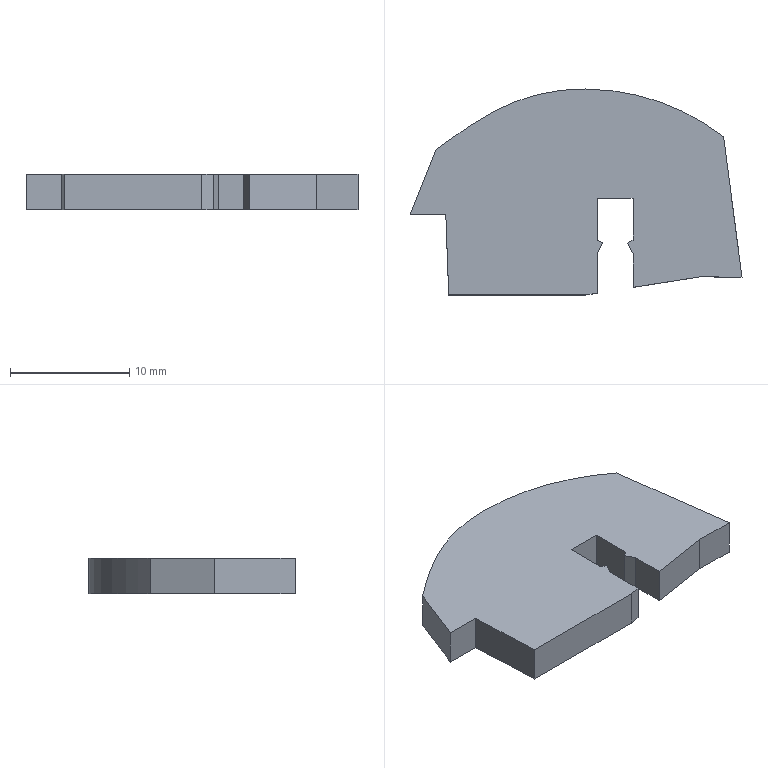Part | SolidWorks | features BaseBody 1 | 1 solid | 21 faces | box 27.839 x 17.276 x 3 mm | volume 1069 mm3 | plane 13 | spline 8
STEP:
#1=CARTESIAN_POINT('',(9.27,15.287,-1.5));
#2=VERTEX_POINT('',#1);
#3=CARTESIAN_POINT('',(-0.006107,19.138,-1.5));
#4=VERTEX_POINT('',#3);
#5=CARTESIAN_POINT('',(9.27,15.287,-1.5));
#6=CARTESIAN_POINT('',(6.696,17.285,-1.5));
#7=CARTESIAN_POINT('',(3.539,18.688,-1.5));
#8=CARTESIAN_POINT('',(-0.006107,19.138,-1.5));
#9=B_SPLINE_CURVE_WITH_KNOTS('',3,(#5,#6,#7,#8),.UNSPECIFIED.,.F.,.F.,(4,4),(0.9,1.),.UNSPECIFIED.);
#10=EDGE_CURVE('',#2,#4,#9,.T.);
#11=ORIENTED_EDGE('',*,*,#10,.F.);
#12=CARTESIAN_POINT('',(10.816,3.504,-1.5));
#13=VERTEX_POINT('',#12);
#14=CARTESIAN_POINT('',(10.816,3.504,-1.5));
#15=CARTESIAN_POINT('',(9.799,11.355,-1.5));
#16=CARTESIAN_POINT('',(9.27,15.287,-1.5));
#17=B_SPLINE_CURVE_WITH_KNOTS('',2,(#14,#15,#16),.UNSPECIFIED.,.F.,.F.,(3,3),(0.85,0.9),.UNSPECIFIED.);
#18=EDGE_CURVE('',#13,#2,#17,.T.);
#19=ORIENTED_EDGE('',*,*,#18,.F.);
#20=CARTESIAN_POINT('',(7.333,3.55,-1.5));
#21=VERTEX_POINT('',#20);
#22=CARTESIAN_POINT('',(7.333,3.55,-1.5));
#23=CARTESIAN_POINT('',(8.52,3.533,-1.5));
#24=CARTESIAN_POINT('',(10.816,3.504,-1.5));
#25=B_SPLINE_CURVE_WITH_KNOTS('',2,(#22,#23,#24),.UNSPECIFIED.,.F.,.F.,(3,3),(0.8,0.85),.UNSPECIFIED.);
#26=EDGE_CURVE('',#21,#13,#25,.T.);
#27=ORIENTED_EDGE('',*,*,#26,.F.);
#28=CARTESIAN_POINT('',(1.678,2.665,-1.5));
#29=VERTEX_POINT('',#28);
#30=CARTESIAN_POINT('',(1.678,2.665,-1.5));
#31=CARTESIAN_POINT('',(5.448,3.256,-1.5));
#32=CARTESIAN_POINT('',(7.333,3.55,-1.5));
#33=B_SPLINE_CURVE_WITH_KNOTS('',2,(#30,#31,#32),.UNSPECIFIED.,.F.,.F.,(3,3),(0.75,0.8),.UNSPECIFIED.);
#34=EDGE_CURVE('',#29,#21,#33,.T.);
#35=ORIENTED_EDGE('',*,*,#34,.F.);
#36=CARTESIAN_POINT('',(1.678,5.468,-1.5));
#37=VERTEX_POINT('',#36);
#38=CARTESIAN_POINT('',(1.678,5.468,-1.5));
#39=DIRECTION('',(0.,-1.,0.));
#40=VECTOR('',#39,1000.);
#41=LINE('',#38,#40);
#42=EDGE_CURVE('',#37,#29,#41,.T.);
#43=ORIENTED_EDGE('',*,*,#42,.F.);
#44=CARTESIAN_POINT('',(1.228,6.361,-1.5));
#45=VERTEX_POINT('',#44);
#46=CARTESIAN_POINT('',(1.228,6.361,-1.5));
#47=DIRECTION('',(0.4506,-0.8927,0.));
#48=VECTOR('',#47,1000.);
#49=LINE('',#46,#48);
#50=EDGE_CURVE('',#45,#37,#49,.T.);
#51=ORIENTED_EDGE('',*,*,#50,.F.);
#52=CARTESIAN_POINT('',(1.678,6.624,-1.5));
#53=VERTEX_POINT('',#52);
#54=CARTESIAN_POINT('',(1.678,6.624,-1.5));
#55=DIRECTION('',(-0.8634,-0.5045,0.));
#56=VECTOR('',#55,1000.);
#57=LINE('',#54,#56);
#58=EDGE_CURVE('',#53,#45,#57,.T.);
#59=ORIENTED_EDGE('',*,*,#58,.F.);
#60=CARTESIAN_POINT('',(1.678,10.134,-1.5));
#61=VERTEX_POINT('',#60);
#62=CARTESIAN_POINT('',(1.678,10.134,-1.5));
#63=DIRECTION('',(0.,-1.,0.));
#64=VECTOR('',#63,1000.);
#65=LINE('',#62,#64);
#66=EDGE_CURVE('',#61,#53,#65,.T.);
#67=ORIENTED_EDGE('',*,*,#66,.F.);
#68=CARTESIAN_POINT('',(-1.319,10.134,-1.5));
#69=VERTEX_POINT('',#68);
#70=CARTESIAN_POINT('',(-1.319,10.134,-1.5));
#71=DIRECTION('',(1.,0.,0.));
#72=VECTOR('',#71,1000.);
#73=LINE('',#70,#72);
#74=EDGE_CURVE('',#69,#61,#73,.T.);
#75=ORIENTED_EDGE('',*,*,#74,.F.);
#76=CARTESIAN_POINT('',(-1.319,6.624,-1.5));
#77=VERTEX_POINT('',#76);
#78=CARTESIAN_POINT('',(-1.319,6.624,-1.5));
#79=DIRECTION('',(0.,1.,0.));
#80=VECTOR('',#79,1000.);
#81=LINE('',#78,#80);
#82=EDGE_CURVE('',#77,#69,#81,.T.);
#83=ORIENTED_EDGE('',*,*,#82,.F.);
#84=CARTESIAN_POINT('',(-0.8705,6.393,-1.5));
#85=VERTEX_POINT('',#84);
#86=CARTESIAN_POINT('',(-0.8705,6.393,-1.5));
#87=DIRECTION('',(-0.8897,0.4565,0.));
#88=VECTOR('',#87,1000.);
#89=LINE('',#86,#88);
#90=EDGE_CURVE('',#85,#77,#89,.T.);
#91=ORIENTED_EDGE('',*,*,#90,.F.);
#92=CARTESIAN_POINT('',(-1.319,5.468,-1.5));
#93=VERTEX_POINT('',#92);
#94=CARTESIAN_POINT('',(-1.319,5.468,-1.5));
#95=DIRECTION('',(0.4365,0.8997,0.));
#96=VECTOR('',#95,1000.);
#97=LINE('',#94,#96);
#98=EDGE_CURVE('',#93,#85,#97,.T.);
#99=ORIENTED_EDGE('',*,*,#98,.F.);
#100=CARTESIAN_POINT('',(-1.319,2.18,-1.5));
#101=VERTEX_POINT('',#100);
#102=CARTESIAN_POINT('',(-1.319,2.18,-1.5));
#103=DIRECTION('',(0.,1.,0.));
#104=VECTOR('',#103,1000.);
#105=LINE('',#102,#104);
#106=EDGE_CURVE('',#101,#93,#105,.T.);
#107=ORIENTED_EDGE('',*,*,#106,.F.);
#108=CARTESIAN_POINT('',(-2.279,2.022,-1.5));
#109=VERTEX_POINT('',#108);
#110=CARTESIAN_POINT('',(-2.279,2.022,-1.5));
#111=CARTESIAN_POINT('',(-1.959,2.076,-1.5));
#112=CARTESIAN_POINT('',(-1.319,2.18,-1.5));
#113=B_SPLINE_CURVE_WITH_KNOTS('',2,(#110,#111,#112),.UNSPECIFIED.,.F.,.F.,(3,3),(0.25,0.3),.UNSPECIFIED.);
#114=EDGE_CURVE('',#109,#101,#113,.T.);
#115=ORIENTED_EDGE('',*,*,#114,.F.);
#116=CARTESIAN_POINT('',(-13.778,2.022,-1.5));
#117=VERTEX_POINT('',#116);
#118=CARTESIAN_POINT('',(-13.778,2.022,-1.5));
#119=DIRECTION('',(1.,0.,0.));
#120=VECTOR('',#119,1000.);
#121=LINE('',#118,#120);
#122=EDGE_CURVE('',#117,#109,#121,.T.);
#123=ORIENTED_EDGE('',*,*,#122,.F.);
#124=CARTESIAN_POINT('',(-14.022,8.734,-1.5));
#125=VERTEX_POINT('',#124);
#126=CARTESIAN_POINT('',(-14.022,8.734,-1.5));
#127=CARTESIAN_POINT('',(-13.939,6.499,-1.5));
#128=CARTESIAN_POINT('',(-13.858,4.261,-1.5));
#129=CARTESIAN_POINT('',(-13.778,2.022,-1.5));
#130=B_SPLINE_CURVE_WITH_KNOTS('',3,(#126,#127,#128,#129),.UNSPECIFIED.,.F.,.F.,(4,4),(0.15,0.2),.UNSPECIFIED.);
#131=EDGE_CURVE('',#125,#117,#130,.T.);
#132=ORIENTED_EDGE('',*,*,#131,.F.);
#133=CARTESIAN_POINT('',(-17.024,8.734,-1.5));
#134=VERTEX_POINT('',#133);
#135=CARTESIAN_POINT('',(-17.024,8.734,-1.5));
#136=DIRECTION('',(1.,0.,0.));
#137=VECTOR('',#136,1000.);
#138=LINE('',#135,#137);
#139=EDGE_CURVE('',#134,#125,#138,.T.);
#140=ORIENTED_EDGE('',*,*,#139,.F.);
#141=CARTESIAN_POINT('',(-14.868,14.173,-1.5));
#142=VERTEX_POINT('',#141);
#143=CARTESIAN_POINT('',(-14.868,14.173,-1.5));
#144=CARTESIAN_POINT('',(-15.587,12.359,-1.5));
#145=CARTESIAN_POINT('',(-16.305,10.548,-1.5));
#146=CARTESIAN_POINT('',(-17.024,8.734,-1.5));
#147=B_SPLINE_CURVE_WITH_KNOTS('',3,(#143,#144,#145,#146),.UNSPECIFIED.,.F.,.F.,(4,4),(0.05,0.1),.UNSPECIFIED.);
#148=EDGE_CURVE('',#142,#134,#147,.T.);
#149=ORIENTED_EDGE('',*,*,#148,.F.);
#150=CARTESIAN_POINT('',(-0.006107,19.138,-1.5));
#151=CARTESIAN_POINT('',(-6.949,20.02,-1.5));
#152=CARTESIAN_POINT('',(-10.909,17.098,-1.5));
#153=CARTESIAN_POINT('',(-14.868,14.173,-1.5));
#154=B_SPLINE_CURVE_WITH_KNOTS('',3,(#150,#151,#152,#153),.UNSPECIFIED.,.F.,.F.,(4,4),(0.,0.05),.UNSPECIFIED.);
#155=EDGE_CURVE('',#4,#142,#154,.T.);
#156=ORIENTED_EDGE('',*,*,#155,.F.);
#157=EDGE_LOOP('',(#11,#19,#27,#35,#43,#51,#59,#67,#75,#83,#91,#99,#107,#115,#123,#132,#140,#149,#156));
#158=FACE_OUTER_BOUND('',#157,.T.);
#159=CARTESIAN_POINT('',(4.996,17.793,-1.5));
#160=DIRECTION('',(0.,0.,-1.));
#161=DIRECTION('',(0.,-1.,0.));
#162=AXIS2_PLACEMENT_3D('',#159,#160,#161);
#163=PLANE('',#162);
#164=ADVANCED_FACE('',(#158),#163,.T.);
#165=CARTESIAN_POINT('',(9.27,15.287,1.5));
#166=VERTEX_POINT('',#165);
#167=CARTESIAN_POINT('',(-0.006107,19.138,1.5));
#168=VERTEX_POINT('',#167);
#169=CARTESIAN_POINT('',(9.27,15.287,1.5));
#170=CARTESIAN_POINT('',(6.696,17.285,1.5));
#171=CARTESIAN_POINT('',(3.539,18.688,1.5));
#172=CARTESIAN_POINT('',(-0.006107,19.138,1.5));
#173=B_SPLINE_CURVE_WITH_KNOTS('',3,(#169,#170,#171,#172),.UNSPECIFIED.,.F.,.F.,(4,4),(0.9,1.),.UNSPECIFIED.);
#174=EDGE_CURVE('',#166,#168,#173,.T.);
#175=ORIENTED_EDGE('',*,*,#174,.T.);
#176=CARTESIAN_POINT('',(-14.868,14.173,1.5));
#177=VERTEX_POINT('',#176);
#178=CARTESIAN_POINT('',(-0.006107,19.138,1.5));
#179=CARTESIAN_POINT('',(-6.949,20.02,1.5));
#180=CARTESIAN_POINT('',(-10.909,17.098,1.5));
#181=CARTESIAN_POINT('',(-14.868,14.173,1.5));
#182=B_SPLINE_CURVE_WITH_KNOTS('',3,(#178,#179,#180,#181),.UNSPECIFIED.,.F.,.F.,(4,4),(0.,0.05),.UNSPECIFIED.);
#183=EDGE_CURVE('',#168,#177,#182,.T.);
#184=ORIENTED_EDGE('',*,*,#183,.T.);
#185=CARTESIAN_POINT('',(-17.024,8.734,1.5));
#186=VERTEX_POINT('',#185);
#187=CARTESIAN_POINT('',(-14.868,14.173,1.5));
#188=CARTESIAN_POINT('',(-15.587,12.359,1.5));
#189=CARTESIAN_POINT('',(-16.305,10.548,1.5));
#190=CARTESIAN_POINT('',(-17.024,8.734,1.5));
#191=B_SPLINE_CURVE_WITH_KNOTS('',3,(#187,#188,#189,#190),.UNSPECIFIED.,.F.,.F.,(4,4),(0.05,0.1),.UNSPECIFIED.);
#192=EDGE_CURVE('',#177,#186,#191,.T.);
#193=ORIENTED_EDGE('',*,*,#192,.T.);
#194=CARTESIAN_POINT('',(-14.022,8.734,1.5));
#195=VERTEX_POINT('',#194);
#196=CARTESIAN_POINT('',(-17.024,8.734,1.5));
#197=DIRECTION('',(1.,0.,0.));
#198=VECTOR('',#197,1000.);
#199=LINE('',#196,#198);
#200=EDGE_CURVE('',#186,#195,#199,.T.);
#201=ORIENTED_EDGE('',*,*,#200,.T.);
#202=CARTESIAN_POINT('',(-13.778,2.022,1.5));
#203=VERTEX_POINT('',#202);
#204=CARTESIAN_POINT('',(-14.022,8.734,1.5));
#205=CARTESIAN_POINT('',(-13.939,6.499,1.5));
#206=CARTESIAN_POINT('',(-13.858,4.261,1.5));
#207=CARTESIAN_POINT('',(-13.778,2.022,1.5));
#208=B_SPLINE_CURVE_WITH_KNOTS('',3,(#204,#205,#206,#207),.UNSPECIFIED.,.F.,.F.,(4,4),(0.15,0.2),.UNSPECIFIED.);
#209=EDGE_CURVE('',#195,#203,#208,.T.);
#210=ORIENTED_EDGE('',*,*,#209,.T.);
#211=CARTESIAN_POINT('',(-2.279,2.022,1.5));
#212=VERTEX_POINT('',#211);
#213=CARTESIAN_POINT('',(-13.778,2.022,1.5));
#214=DIRECTION('',(1.,0.,0.));
#215=VECTOR('',#214,1000.);
#216=LINE('',#213,#215);
#217=EDGE_CURVE('',#203,#212,#216,.T.);
#218=ORIENTED_EDGE('',*,*,#217,.T.);
#219=CARTESIAN_POINT('',(-1.319,2.18,1.5));
#220=VERTEX_POINT('',#219);
#221=CARTESIAN_POINT('',(-2.279,2.022,1.5));
#222=CARTESIAN_POINT('',(-1.959,2.076,1.5));
#223=CARTESIAN_POINT('',(-1.319,2.18,1.5));
#224=B_SPLINE_CURVE_WITH_KNOTS('',2,(#221,#222,#223),.UNSPECIFIED.,.F.,.F.,(3,3),(0.25,0.3),.UNSPECIFIED.);
#225=EDGE_CURVE('',#212,#220,#224,.T.);
#226=ORIENTED_EDGE('',*,*,#225,.T.);
#227=CARTESIAN_POINT('',(-1.319,5.468,1.5));
#228=VERTEX_POINT('',#227);
#229=CARTESIAN_POINT('',(-1.319,2.18,1.5));
#230=DIRECTION('',(0.,1.,0.));
#231=VECTOR('',#230,1000.);
#232=LINE('',#229,#231);
#233=EDGE_CURVE('',#220,#228,#232,.T.);
#234=ORIENTED_EDGE('',*,*,#233,.T.);
#235=CARTESIAN_POINT('',(-0.8705,6.393,1.5));
#236=VERTEX_POINT('',#235);
#237=CARTESIAN_POINT('',(-1.319,5.468,1.5));
#238=DIRECTION('',(0.4365,0.8997,0.));
#239=VECTOR('',#238,1000.);
#240=LINE('',#237,#239);
#241=EDGE_CURVE('',#228,#236,#240,.T.);
#242=ORIENTED_EDGE('',*,*,#241,.T.);
#243=CARTESIAN_POINT('',(-1.319,6.624,1.5));
#244=VERTEX_POINT('',#243);
#245=CARTESIAN_POINT('',(-0.8705,6.393,1.5));
#246=DIRECTION('',(-0.8897,0.4565,0.));
#247=VECTOR('',#246,1000.);
#248=LINE('',#245,#247);
#249=EDGE_CURVE('',#236,#244,#248,.T.);
#250=ORIENTED_EDGE('',*,*,#249,.T.);
#251=CARTESIAN_POINT('',(-1.319,10.134,1.5));
#252=VERTEX_POINT('',#251);
#253=CARTESIAN_POINT('',(-1.319,6.624,1.5));
#254=DIRECTION('',(0.,1.,0.));
#255=VECTOR('',#254,1000.);
#256=LINE('',#253,#255);
#257=EDGE_CURVE('',#244,#252,#256,.T.);
#258=ORIENTED_EDGE('',*,*,#257,.T.);
#259=CARTESIAN_POINT('',(1.678,10.134,1.5));
#260=VERTEX_POINT('',#259);
#261=CARTESIAN_POINT('',(-1.319,10.134,1.5));
#262=DIRECTION('',(1.,0.,0.));
#263=VECTOR('',#262,1000.);
#264=LINE('',#261,#263);
#265=EDGE_CURVE('',#252,#260,#264,.T.);
#266=ORIENTED_EDGE('',*,*,#265,.T.);
#267=CARTESIAN_POINT('',(1.678,6.624,1.5));
#268=VERTEX_POINT('',#267);
#269=CARTESIAN_POINT('',(1.678,10.134,1.5));
#270=DIRECTION('',(0.,-1.,0.));
#271=VECTOR('',#270,1000.);
#272=LINE('',#269,#271);
#273=EDGE_CURVE('',#260,#268,#272,.T.);
#274=ORIENTED_EDGE('',*,*,#273,.T.);
#275=CARTESIAN_POINT('',(1.228,6.361,1.5));
#276=VERTEX_POINT('',#275);
#277=CARTESIAN_POINT('',(1.678,6.624,1.5));
#278=DIRECTION('',(-0.8634,-0.5045,0.));
#279=VECTOR('',#278,1000.);
#280=LINE('',#277,#279);
#281=EDGE_CURVE('',#268,#276,#280,.T.);
#282=ORIENTED_EDGE('',*,*,#281,.T.);
#283=CARTESIAN_POINT('',(1.678,5.468,1.5));
#284=VERTEX_POINT('',#283);
#285=CARTESIAN_POINT('',(1.228,6.361,1.5));
#286=DIRECTION('',(0.4506,-0.8927,0.));
#287=VECTOR('',#286,1000.);
#288=LINE('',#285,#287);
#289=EDGE_CURVE('',#276,#284,#288,.T.);
#290=ORIENTED_EDGE('',*,*,#289,.T.);
#291=CARTESIAN_POINT('',(1.678,2.665,1.5));
#292=VERTEX_POINT('',#291);
#293=CARTESIAN_POINT('',(1.678,5.468,1.5));
#294=DIRECTION('',(0.,-1.,0.));
#295=VECTOR('',#294,1000.);
#296=LINE('',#293,#295);
#297=EDGE_CURVE('',#284,#292,#296,.T.);
#298=ORIENTED_EDGE('',*,*,#297,.T.);
#299=CARTESIAN_POINT('',(7.333,3.55,1.5));
#300=VERTEX_POINT('',#299);
#301=CARTESIAN_POINT('',(1.678,2.665,1.5));
#302=CARTESIAN_POINT('',(5.448,3.256,1.5));
#303=CARTESIAN_POINT('',(7.333,3.55,1.5));
#304=B_SPLINE_CURVE_WITH_KNOTS('',2,(#301,#302,#303),.UNSPECIFIED.,.F.,.F.,(3,3),(0.75,0.8),.UNSPECIFIED.);
#305=EDGE_CURVE('',#292,#300,#304,.T.);
#306=ORIENTED_EDGE('',*,*,#305,.T.);
#307=CARTESIAN_POINT('',(10.816,3.504,1.5));
#308=VERTEX_POINT('',#307);
#309=CARTESIAN_POINT('',(7.333,3.55,1.5));
#310=CARTESIAN_POINT('',(8.52,3.533,1.5));
#311=CARTESIAN_POINT('',(10.816,3.504,1.5));
#312=B_SPLINE_CURVE_WITH_KNOTS('',2,(#309,#310,#311),.UNSPECIFIED.,.F.,.F.,(3,3),(0.8,0.85),.UNSPECIFIED.);
#313=EDGE_CURVE('',#300,#308,#312,.T.);
#314=ORIENTED_EDGE('',*,*,#313,.T.);
#315=CARTESIAN_POINT('',(10.816,3.504,1.5));
#316=CARTESIAN_POINT('',(9.799,11.355,1.5));
#317=CARTESIAN_POINT('',(9.27,15.287,1.5));
#318=B_SPLINE_CURVE_WITH_KNOTS('',2,(#315,#316,#317),.UNSPECIFIED.,.F.,.F.,(3,3),(0.85,0.9),.UNSPECIFIED.);
#319=EDGE_CURVE('',#308,#166,#318,.T.);
#320=ORIENTED_EDGE('',*,*,#319,.T.);
#321=EDGE_LOOP('',(#175,#184,#193,#201,#210,#218,#226,#234,#242,#250,#258,#266,#274,#282,#290,#298,#306,#314,#320));
#322=FACE_OUTER_BOUND('',#321,.T.);
#323=CARTESIAN_POINT('',(4.996,17.793,1.5));
#324=DIRECTION('',(0.,0.,-1.));
#325=DIRECTION('',(0.,-1.,0.));
#326=AXIS2_PLACEMENT_3D('',#323,#324,#325);
#327=PLANE('',#326);
#328=ADVANCED_FACE('',(#322),#327,.F.);
#329=ORIENTED_EDGE('',*,*,#18,.T.);
#330=CARTESIAN_POINT('',(9.27,15.287,1.5));
#331=DIRECTION('',(0.,0.,-1.));
#332=VECTOR('',#331,1000.);
#333=LINE('',#330,#332);
#334=EDGE_CURVE('',#166,#2,#333,.T.);
#335=ORIENTED_EDGE('',*,*,#334,.F.);
#336=ORIENTED_EDGE('',*,*,#319,.F.);
#337=CARTESIAN_POINT('',(10.816,3.504,1.5));
#338=DIRECTION('',(0.,0.,-1.));
#339=VECTOR('',#338,1000.);
#340=LINE('',#337,#339);
#341=EDGE_CURVE('',#308,#13,#340,.T.);
#342=ORIENTED_EDGE('',*,*,#341,.T.);
#343=EDGE_LOOP('',(#329,#335,#336,#342));
#344=FACE_OUTER_BOUND('',#343,.T.);
#345=CARTESIAN_POINT('',(10.816,3.504,1.5));
#346=CARTESIAN_POINT('',(10.816,3.504,-1.5));
#347=CARTESIAN_POINT('',(9.799,11.355,1.5));
#348=CARTESIAN_POINT('',(9.799,11.355,-1.5));
#349=CARTESIAN_POINT('',(9.27,15.287,1.5));
#350=CARTESIAN_POINT('',(9.27,15.287,-1.5));
#351=B_SPLINE_SURFACE_WITH_KNOTS('',2,1,((#345,#346),(#347,#348),(#349,#350)),.UNSPECIFIED.,.F.,.F.,.F.,(3,3),(2,2),(0.85,0.9),(0.,1.),.UNSPECIFIED.);
#352=ADVANCED_FACE('',(#344),#351,.F.);
#353=ORIENTED_EDGE('',*,*,#26,.T.);
#354=ORIENTED_EDGE('',*,*,#341,.F.);
#355=ORIENTED_EDGE('',*,*,#313,.F.);
#356=CARTESIAN_POINT('',(7.333,3.55,1.5));
#357=DIRECTION('',(0.,0.,-1.));
#358=VECTOR('',#357,1000.);
#359=LINE('',#356,#358);
#360=EDGE_CURVE('',#300,#21,#359,.T.);
#361=ORIENTED_EDGE('',*,*,#360,.T.);
#362=EDGE_LOOP('',(#353,#354,#355,#361));
#363=FACE_OUTER_BOUND('',#362,.T.);
#364=CARTESIAN_POINT('',(7.333,3.55,1.5));
#365=CARTESIAN_POINT('',(7.333,3.55,-1.5));
#366=CARTESIAN_POINT('',(8.52,3.533,1.5));
#367=CARTESIAN_POINT('',(8.52,3.533,-1.5));
#368=CARTESIAN_POINT('',(10.816,3.504,1.5));
#369=CARTESIAN_POINT('',(10.816,3.504,-1.5));
#370=B_SPLINE_SURFACE_WITH_KNOTS('',2,1,((#364,#365),(#366,#367),(#368,#369)),.UNSPECIFIED.,.F.,.F.,.F.,(3,3),(2,2),(0.8,0.85),(0.,1.),.UNSPECIFIED.);
#371=ADVANCED_FACE('',(#363),#370,.F.);
#372=ORIENTED_EDGE('',*,*,#34,.T.);
#373=ORIENTED_EDGE('',*,*,#360,.F.);
#374=ORIENTED_EDGE('',*,*,#305,.F.);
#375=CARTESIAN_POINT('',(1.678,2.665,1.5));
#376=DIRECTION('',(0.,0.,-1.));
#377=VECTOR('',#376,1000.);
#378=LINE('',#375,#377);
#379=EDGE_CURVE('',#292,#29,#378,.T.);
#380=ORIENTED_EDGE('',*,*,#379,.T.);
#381=EDGE_LOOP('',(#372,#373,#374,#380));
#382=FACE_OUTER_BOUND('',#381,.T.);
#383=CARTESIAN_POINT('',(1.678,2.665,1.5));
#384=CARTESIAN_POINT('',(1.678,2.665,-1.5));
#385=CARTESIAN_POINT('',(5.448,3.256,1.5));
#386=CARTESIAN_POINT('',(5.448,3.256,-1.5));
#387=CARTESIAN_POINT('',(7.333,3.55,1.5));
#388=CARTESIAN_POINT('',(7.333,3.55,-1.5));
#389=B_SPLINE_SURFACE_WITH_KNOTS('',2,1,((#383,#384),(#385,#386),(#387,#388)),.UNSPECIFIED.,.F.,.F.,.F.,(3,3),(2,2),(0.75,0.8),(0.,1.),.UNSPECIFIED.);
#390=ADVANCED_FACE('',(#382),#389,.F.);
#391=ORIENTED_EDGE('',*,*,#42,.T.);
#392=ORIENTED_EDGE('',*,*,#379,.F.);
#393=ORIENTED_EDGE('',*,*,#297,.F.);
#394=CARTESIAN_POINT('',(1.678,5.468,1.5));
#395=DIRECTION('',(0.,0.,-1.));
#396=VECTOR('',#395,1000.);
#397=LINE('',#394,#396);
#398=EDGE_CURVE('',#284,#37,#397,.T.);
#399=ORIENTED_EDGE('',*,*,#398,.T.);
#400=EDGE_LOOP('',(#391,#392,#393,#399));
#401=FACE_OUTER_BOUND('',#400,.T.);
#402=CARTESIAN_POINT('',(1.678,5.468,1.5));
#403=DIRECTION('',(1.,0.,0.));
#404=DIRECTION('',(0.,1.,0.));
#405=AXIS2_PLACEMENT_3D('',#402,#403,#404);
#406=PLANE('',#405);
#407=ADVANCED_FACE('',(#401),#406,.F.);
#408=ORIENTED_EDGE('',*,*,#50,.T.);
#409=ORIENTED_EDGE('',*,*,#398,.F.);
#410=ORIENTED_EDGE('',*,*,#289,.F.);
#411=CARTESIAN_POINT('',(1.228,6.361,1.5));
#412=DIRECTION('',(0.,0.,-1.));
#413=VECTOR('',#412,1000.);
#414=LINE('',#411,#413);
#415=EDGE_CURVE('',#276,#45,#414,.T.);
#416=ORIENTED_EDGE('',*,*,#415,.T.);
#417=EDGE_LOOP('',(#408,#409,#410,#416));
#418=FACE_OUTER_BOUND('',#417,.T.);
#419=CARTESIAN_POINT('',(1.228,6.361,1.5));
#420=DIRECTION('',(0.8927,0.4506,0.));
#421=DIRECTION('',(0.,0.,-1.));
#422=AXIS2_PLACEMENT_3D('',#419,#420,#421);
#423=PLANE('',#422);
#424=ADVANCED_FACE('',(#418),#423,.F.);
#425=ORIENTED_EDGE('',*,*,#58,.T.);
#426=ORIENTED_EDGE('',*,*,#415,.F.);
#427=ORIENTED_EDGE('',*,*,#281,.F.);
#428=CARTESIAN_POINT('',(1.678,6.624,1.5));
#429=DIRECTION('',(0.,0.,-1.));
#430=VECTOR('',#429,1000.);
#431=LINE('',#428,#430);
#432=EDGE_CURVE('',#268,#53,#431,.T.);
#433=ORIENTED_EDGE('',*,*,#432,.T.);
#434=EDGE_LOOP('',(#425,#426,#427,#433));
#435=FACE_OUTER_BOUND('',#434,.T.);
#436=CARTESIAN_POINT('',(1.678,6.624,1.5));
#437=DIRECTION('',(0.5045,-0.8634,0.));
#438=DIRECTION('',(0.,0.,-1.));
#439=AXIS2_PLACEMENT_3D('',#436,#437,#438);
#440=PLANE('',#439);
#441=ADVANCED_FACE('',(#435),#440,.F.);
#442=ORIENTED_EDGE('',*,*,#66,.T.);
#443=ORIENTED_EDGE('',*,*,#432,.F.);
#444=ORIENTED_EDGE('',*,*,#273,.F.);
#445=CARTESIAN_POINT('',(1.678,10.134,1.5));
#446=DIRECTION('',(0.,0.,-1.));
#447=VECTOR('',#446,1000.);
#448=LINE('',#445,#447);
#449=EDGE_CURVE('',#260,#61,#448,.T.);
#450=ORIENTED_EDGE('',*,*,#449,.T.);
#451=EDGE_LOOP('',(#442,#443,#444,#450));
#452=FACE_OUTER_BOUND('',#451,.T.);
#453=CARTESIAN_POINT('',(1.678,10.134,1.5));
#454=DIRECTION('',(1.,0.,0.));
#455=DIRECTION('',(0.,1.,0.));
#456=AXIS2_PLACEMENT_3D('',#453,#454,#455);
#457=PLANE('',#456);
#458=ADVANCED_FACE('',(#452),#457,.F.);
#459=ORIENTED_EDGE('',*,*,#74,.T.);
#460=ORIENTED_EDGE('',*,*,#449,.F.);
#461=ORIENTED_EDGE('',*,*,#265,.F.);
#462=CARTESIAN_POINT('',(-1.319,10.134,1.5));
#463=DIRECTION('',(0.,0.,-1.));
#464=VECTOR('',#463,1000.);
#465=LINE('',#462,#464);
#466=EDGE_CURVE('',#252,#69,#465,.T.);
#467=ORIENTED_EDGE('',*,*,#466,.T.);
#468=EDGE_LOOP('',(#459,#460,#461,#467));
#469=FACE_OUTER_BOUND('',#468,.T.);
#470=CARTESIAN_POINT('',(-1.319,10.134,1.5));
#471=DIRECTION('',(0.,1.,0.));
#472=DIRECTION('',(1.,0.,0.));
#473=AXIS2_PLACEMENT_3D('',#470,#471,#472);
#474=PLANE('',#473);
#475=ADVANCED_FACE('',(#469),#474,.F.);
#476=ORIENTED_EDGE('',*,*,#82,.T.);
#477=ORIENTED_EDGE('',*,*,#466,.F.);
#478=ORIENTED_EDGE('',*,*,#257,.F.);
#479=CARTESIAN_POINT('',(-1.319,6.624,1.5));
#480=DIRECTION('',(0.,0.,-1.));
#481=VECTOR('',#480,1000.);
#482=LINE('',#479,#481);
#483=EDGE_CURVE('',#244,#77,#482,.T.);
#484=ORIENTED_EDGE('',*,*,#483,.T.);
#485=EDGE_LOOP('',(#476,#477,#478,#484));
#486=FACE_OUTER_BOUND('',#485,.T.);
#487=CARTESIAN_POINT('',(-1.319,6.624,1.5));
#488=DIRECTION('',(-1.,0.,0.));
#489=DIRECTION('',(0.,0.,1.));
#490=AXIS2_PLACEMENT_3D('',#487,#488,#489);
#491=PLANE('',#490);
#492=ADVANCED_FACE('',(#486),#491,.F.);
#493=ORIENTED_EDGE('',*,*,#90,.T.);
#494=ORIENTED_EDGE('',*,*,#483,.F.);
#495=ORIENTED_EDGE('',*,*,#249,.F.);
#496=CARTESIAN_POINT('',(-0.8705,6.393,1.5));
#497=DIRECTION('',(0.,0.,-1.));
#498=VECTOR('',#497,1000.);
#499=LINE('',#496,#498);
#500=EDGE_CURVE('',#236,#85,#499,.T.);
#501=ORIENTED_EDGE('',*,*,#500,.T.);
#502=EDGE_LOOP('',(#493,#494,#495,#501));
#503=FACE_OUTER_BOUND('',#502,.T.);
#504=CARTESIAN_POINT('',(-0.8705,6.393,1.5));
#505=DIRECTION('',(-0.4565,-0.8897,0.));
#506=DIRECTION('',(-0.8897,0.4565,0.));
#507=AXIS2_PLACEMENT_3D('',#504,#505,#506);
#508=PLANE('',#507);
#509=ADVANCED_FACE('',(#503),#508,.F.);
#510=ORIENTED_EDGE('',*,*,#98,.T.);
#511=ORIENTED_EDGE('',*,*,#500,.F.);
#512=ORIENTED_EDGE('',*,*,#241,.F.);
#513=CARTESIAN_POINT('',(-1.319,5.468,1.5));
#514=DIRECTION('',(0.,0.,-1.));
#515=VECTOR('',#514,1000.);
#516=LINE('',#513,#515);
#517=EDGE_CURVE('',#228,#93,#516,.T.);
#518=ORIENTED_EDGE('',*,*,#517,.T.);
#519=EDGE_LOOP('',(#510,#511,#512,#518));
#520=FACE_OUTER_BOUND('',#519,.T.);
#521=CARTESIAN_POINT('',(-1.319,5.468,1.5));
#522=DIRECTION('',(-0.8997,0.4365,0.));
#523=DIRECTION('',(0.,0.,1.));
#524=AXIS2_PLACEMENT_3D('',#521,#522,#523);
#525=PLANE('',#524);
#526=ADVANCED_FACE('',(#520),#525,.F.);
#527=ORIENTED_EDGE('',*,*,#106,.T.);
#528=ORIENTED_EDGE('',*,*,#517,.F.);
#529=ORIENTED_EDGE('',*,*,#233,.F.);
#530=CARTESIAN_POINT('',(-1.319,2.18,1.5));
#531=DIRECTION('',(0.,0.,-1.));
#532=VECTOR('',#531,1000.);
#533=LINE('',#530,#532);
#534=EDGE_CURVE('',#220,#101,#533,.T.);
#535=ORIENTED_EDGE('',*,*,#534,.T.);
#536=EDGE_LOOP('',(#527,#528,#529,#535));
#537=FACE_OUTER_BOUND('',#536,.T.);
#538=CARTESIAN_POINT('',(-1.319,2.18,1.5));
#539=DIRECTION('',(-1.,0.,0.));
#540=DIRECTION('',(0.,0.,1.));
#541=AXIS2_PLACEMENT_3D('',#538,#539,#540);
#542=PLANE('',#541);
#543=ADVANCED_FACE('',(#537),#542,.F.);
#544=ORIENTED_EDGE('',*,*,#114,.T.);
#545=ORIENTED_EDGE('',*,*,#534,.F.);
#546=ORIENTED_EDGE('',*,*,#225,.F.);
#547=CARTESIAN_POINT('',(-2.279,2.022,1.5));
#548=DIRECTION('',(0.,0.,-1.));
#549=VECTOR('',#548,1000.);
#550=LINE('',#547,#549);
#551=EDGE_CURVE('',#212,#109,#550,.T.);
#552=ORIENTED_EDGE('',*,*,#551,.T.);
#553=EDGE_LOOP('',(#544,#545,#546,#552));
#554=FACE_OUTER_BOUND('',#553,.T.);
#555=CARTESIAN_POINT('',(-2.279,2.022,1.5));
#556=CARTESIAN_POINT('',(-2.279,2.022,-1.5));
#557=CARTESIAN_POINT('',(-1.959,2.076,1.5));
#558=CARTESIAN_POINT('',(-1.959,2.076,-1.5));
#559=CARTESIAN_POINT('',(-1.319,2.18,1.5));
#560=CARTESIAN_POINT('',(-1.319,2.18,-1.5));
#561=B_SPLINE_SURFACE_WITH_KNOTS('',2,1,((#555,#556),(#557,#558),(#559,#560)),.UNSPECIFIED.,.F.,.F.,.F.,(3,3),(2,2),(0.25,0.3),(0.,1.),.UNSPECIFIED.);
#562=ADVANCED_FACE('',(#554),#561,.F.);
#563=ORIENTED_EDGE('',*,*,#122,.T.);
#564=ORIENTED_EDGE('',*,*,#551,.F.);
#565=ORIENTED_EDGE('',*,*,#217,.F.);
#566=CARTESIAN_POINT('',(-13.778,2.022,1.5));
#567=DIRECTION('',(0.,0.,-1.));
#568=VECTOR('',#567,1000.);
#569=LINE('',#566,#568);
#570=EDGE_CURVE('',#203,#117,#569,.T.);
#571=ORIENTED_EDGE('',*,*,#570,.T.);
#572=EDGE_LOOP('',(#563,#564,#565,#571));
#573=FACE_OUTER_BOUND('',#572,.T.);
#574=CARTESIAN_POINT('',(-13.778,2.022,1.5));
#575=DIRECTION('',(0.,1.,0.));
#576=DIRECTION('',(1.,0.,0.));
#577=AXIS2_PLACEMENT_3D('',#574,#575,#576);
#578=PLANE('',#577);
#579=ADVANCED_FACE('',(#573),#578,.F.);
#580=ORIENTED_EDGE('',*,*,#131,.T.);
#581=ORIENTED_EDGE('',*,*,#570,.F.);
#582=ORIENTED_EDGE('',*,*,#209,.F.);
#583=CARTESIAN_POINT('',(-14.022,8.734,1.5));
#584=DIRECTION('',(0.,0.,-1.));
#585=VECTOR('',#584,1000.);
#586=LINE('',#583,#585);
#587=EDGE_CURVE('',#195,#125,#586,.T.);
#588=ORIENTED_EDGE('',*,*,#587,.T.);
#589=EDGE_LOOP('',(#580,#581,#582,#588));
#590=FACE_OUTER_BOUND('',#589,.T.);
#591=CARTESIAN_POINT('',(-14.022,8.734,1.5));
#592=CARTESIAN_POINT('',(-14.022,8.734,-1.5));
#593=CARTESIAN_POINT('',(-13.939,6.499,1.5));
#594=CARTESIAN_POINT('',(-13.939,6.499,-1.5));
#595=CARTESIAN_POINT('',(-13.858,4.261,1.5));
#596=CARTESIAN_POINT('',(-13.858,4.261,-1.5));
#597=CARTESIAN_POINT('',(-13.778,2.022,1.5));
#598=CARTESIAN_POINT('',(-13.778,2.022,-1.5));
#599=B_SPLINE_SURFACE_WITH_KNOTS('',3,1,((#591,#592),(#593,#594),(#595,#596),(#597,#598)),.UNSPECIFIED.,.F.,.F.,.F.,(4,4),(2,2),(0.15,0.2),(0.,1.),.UNSPECIFIED.);
#600=ADVANCED_FACE('',(#590),#599,.F.);
#601=ORIENTED_EDGE('',*,*,#139,.T.);
#602=ORIENTED_EDGE('',*,*,#587,.F.);
#603=ORIENTED_EDGE('',*,*,#200,.F.);
#604=CARTESIAN_POINT('',(-17.024,8.734,1.5));
#605=DIRECTION('',(0.,0.,-1.));
#606=VECTOR('',#605,1000.);
#607=LINE('',#604,#606);
#608=EDGE_CURVE('',#186,#134,#607,.T.);
#609=ORIENTED_EDGE('',*,*,#608,.T.);
#610=EDGE_LOOP('',(#601,#602,#603,#609));
#611=FACE_OUTER_BOUND('',#610,.T.);
#612=CARTESIAN_POINT('',(-17.024,8.734,1.5));
#613=DIRECTION('',(0.,1.,0.));
#614=DIRECTION('',(1.,0.,0.));
#615=AXIS2_PLACEMENT_3D('',#612,#613,#614);
#616=PLANE('',#615);
#617=ADVANCED_FACE('',(#611),#616,.F.);
#618=ORIENTED_EDGE('',*,*,#148,.T.);
#619=ORIENTED_EDGE('',*,*,#608,.F.);
#620=ORIENTED_EDGE('',*,*,#192,.F.);
#621=CARTESIAN_POINT('',(-14.868,14.173,1.5));
#622=DIRECTION('',(0.,0.,-1.));
#623=VECTOR('',#622,1000.);
#624=LINE('',#621,#623);
#625=EDGE_CURVE('',#177,#142,#624,.T.);
#626=ORIENTED_EDGE('',*,*,#625,.T.);
#627=EDGE_LOOP('',(#618,#619,#620,#626));
#628=FACE_OUTER_BOUND('',#627,.T.);
#629=CARTESIAN_POINT('',(-14.868,14.173,1.5));
#630=CARTESIAN_POINT('',(-14.868,14.173,-1.5));
#631=CARTESIAN_POINT('',(-15.587,12.359,1.5));
#632=CARTESIAN_POINT('',(-15.587,12.359,-1.5));
#633=CARTESIAN_POINT('',(-16.305,10.548,1.5));
#634=CARTESIAN_POINT('',(-16.305,10.548,-1.5));
#635=CARTESIAN_POINT('',(-17.024,8.734,1.5));
#636=CARTESIAN_POINT('',(-17.024,8.734,-1.5));
#637=B_SPLINE_SURFACE_WITH_KNOTS('',3,1,((#629,#630),(#631,#632),(#633,#634),(#635,#636)),.UNSPECIFIED.,.F.,.F.,.F.,(4,4),(2,2),(0.05,0.1),(0.,1.),.UNSPECIFIED.);
#638=ADVANCED_FACE('',(#628),#637,.F.);
#639=ORIENTED_EDGE('',*,*,#155,.T.);
#640=ORIENTED_EDGE('',*,*,#625,.F.);
#641=ORIENTED_EDGE('',*,*,#183,.F.);
#642=CARTESIAN_POINT('',(-0.006107,19.138,1.5));
#643=DIRECTION('',(0.,0.,-1.));
#644=VECTOR('',#643,1000.);
#645=LINE('',#642,#644);
#646=EDGE_CURVE('',#168,#4,#645,.T.);
#647=ORIENTED_EDGE('',*,*,#646,.T.);
#648=EDGE_LOOP('',(#639,#640,#641,#647));
#649=FACE_OUTER_BOUND('',#648,.T.);
#650=CARTESIAN_POINT('',(-0.006107,19.138,1.5));
#651=CARTESIAN_POINT('',(-0.006107,19.138,-1.5));
#652=CARTESIAN_POINT('',(-6.949,20.02,1.5));
#653=CARTESIAN_POINT('',(-6.949,20.02,-1.5));
#654=CARTESIAN_POINT('',(-10.909,17.098,1.5));
#655=CARTESIAN_POINT('',(-10.909,17.098,-1.5));
#656=CARTESIAN_POINT('',(-14.868,14.173,1.5));
#657=CARTESIAN_POINT('',(-14.868,14.173,-1.5));
#658=B_SPLINE_SURFACE_WITH_KNOTS('',3,1,((#650,#651),(#652,#653),(#654,#655),(#656,#657)),.UNSPECIFIED.,.F.,.F.,.F.,(4,4),(2,2),(0.,0.05),(0.,1.),.UNSPECIFIED.);
#659=ADVANCED_FACE('',(#649),#658,.F.);
#660=ORIENTED_EDGE('',*,*,#10,.T.);
#661=ORIENTED_EDGE('',*,*,#646,.F.);
#662=ORIENTED_EDGE('',*,*,#174,.F.);
#663=ORIENTED_EDGE('',*,*,#334,.T.);
#664=EDGE_LOOP('',(#660,#661,#662,#663));
#665=FACE_OUTER_BOUND('',#664,.T.);
#666=CARTESIAN_POINT('',(9.27,15.287,1.5));
#667=CARTESIAN_POINT('',(9.27,15.287,-1.5));
#668=CARTESIAN_POINT('',(6.696,17.285,1.5));
#669=CARTESIAN_POINT('',(6.696,17.285,-1.5));
#670=CARTESIAN_POINT('',(3.539,18.688,1.5));
#671=CARTESIAN_POINT('',(3.539,18.688,-1.5));
#672=CARTESIAN_POINT('',(-0.006107,19.138,1.5));
#673=CARTESIAN_POINT('',(-0.006107,19.138,-1.5));
#674=B_SPLINE_SURFACE_WITH_KNOTS('',3,1,((#666,#667),(#668,#669),(#670,#671),(#672,#673)),.UNSPECIFIED.,.F.,.F.,.F.,(4,4),(2,2),(0.9,1.),(0.,1.),.UNSPECIFIED.);
#675=ADVANCED_FACE('',(#665),#674,.F.);
#676=CLOSED_SHELL('',(#164,#328,#352,#371,#390,#407,#424,#441,#458,#475,#492,#509,#526,#543,#562,#579,#600,#617,#638,#659,#675));
#677=MANIFOLD_SOLID_BREP('',#676);
#678=CARTESIAN_POINT('',(0.,0.,0.));
#679=DIRECTION('',(0.,0.,1.));
#680=DIRECTION('',(1.,0.,0.));
#681=AXIS2_PLACEMENT_3D('',#678,#679,#680);
#682=(LENGTH_UNIT()NAMED_UNIT(*)SI_UNIT(.MILLI.,.METRE.));
#683=UNCERTAINTY_MEASURE_WITH_UNIT(LENGTH_MEASURE(0.00001),#682,'','');
#684=(NAMED_UNIT(*)PLANE_ANGLE_UNIT()SI_UNIT($,.RADIAN.));
#685=(NAMED_UNIT(*)SI_UNIT($,.STERADIAN.)SOLID_ANGLE_UNIT());
#686=(GEOMETRIC_REPRESENTATION_CONTEXT(3)GLOBAL_UNCERTAINTY_ASSIGNED_CONTEXT((#683))GLOBAL_UNIT_ASSIGNED_CONTEXT((#682,#684,#685))REPRESENTATION_CONTEXT('',''));
#687=ADVANCED_BREP_SHAPE_REPRESENTATION('',(#677,#681),#686);